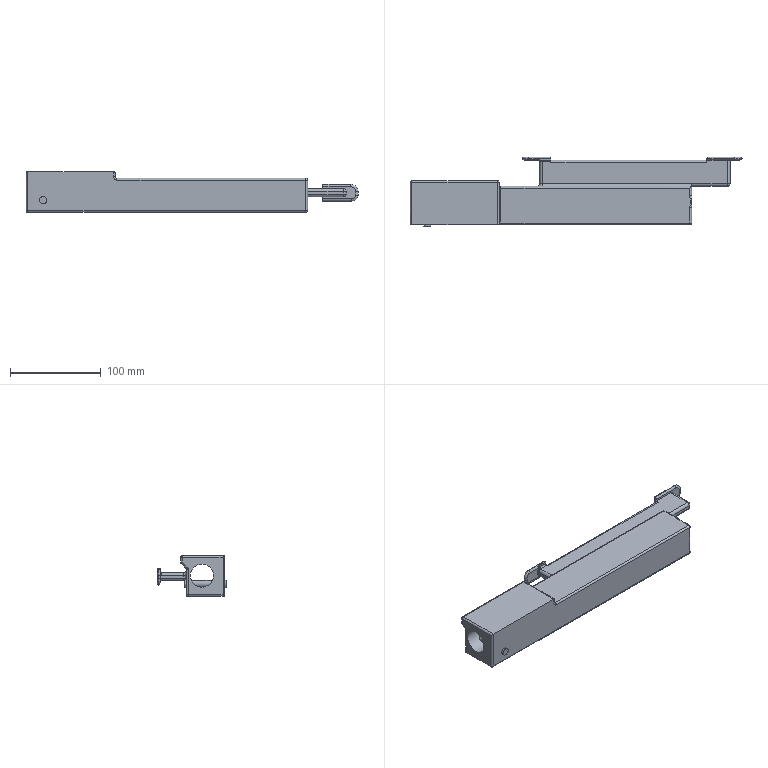Part | STEP file | DEWALT-DWE7492-B22 | 1 solid | 106 faces | box 365.575 x 76.384 x 45 mm | volume 432829 mm3 | cylinder 54 | plane 26 | torus 14 | sphere 10 | spline 2 | commonest cylinder face diameters 4 x23 6 x18 3 x9 8 x3 25.5 x1